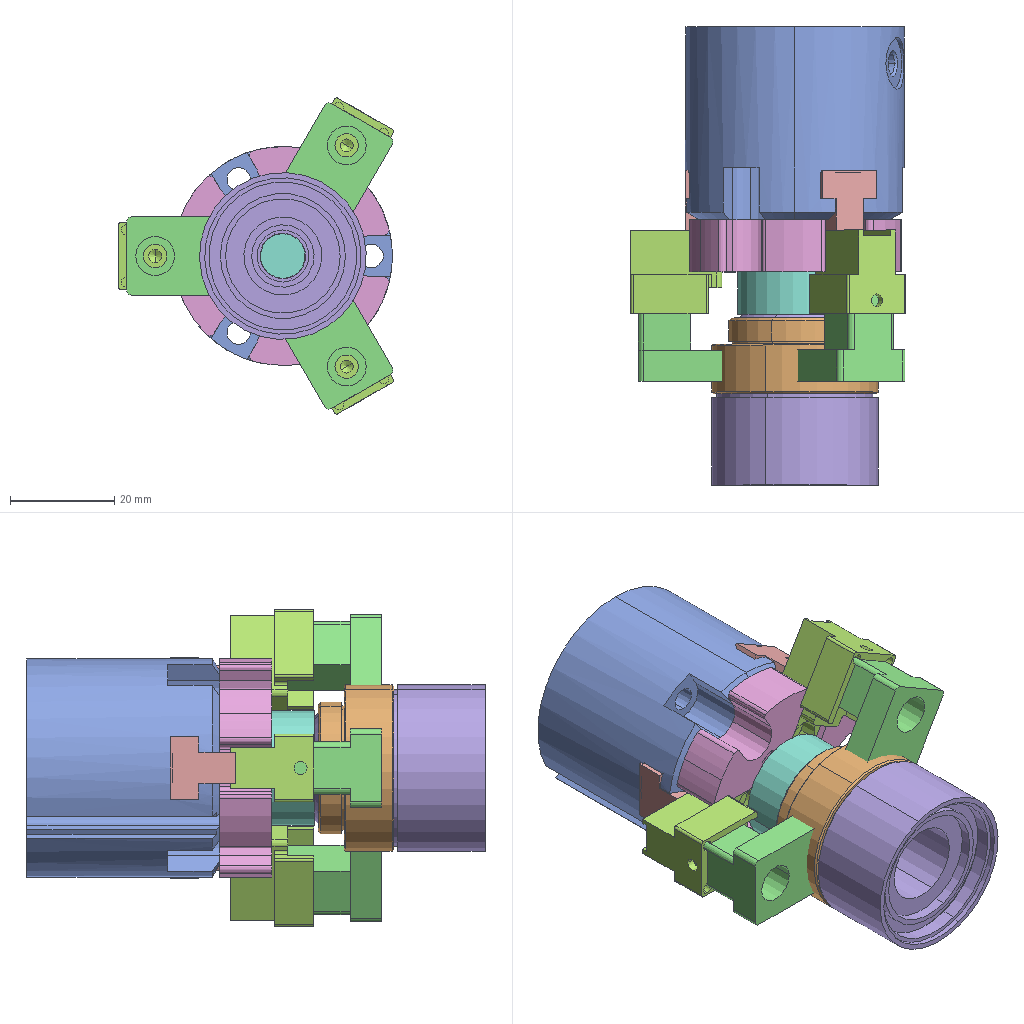Assembly | SolidWorks | 7 different items | 13 placed | box 53 x 88 x 61 mm
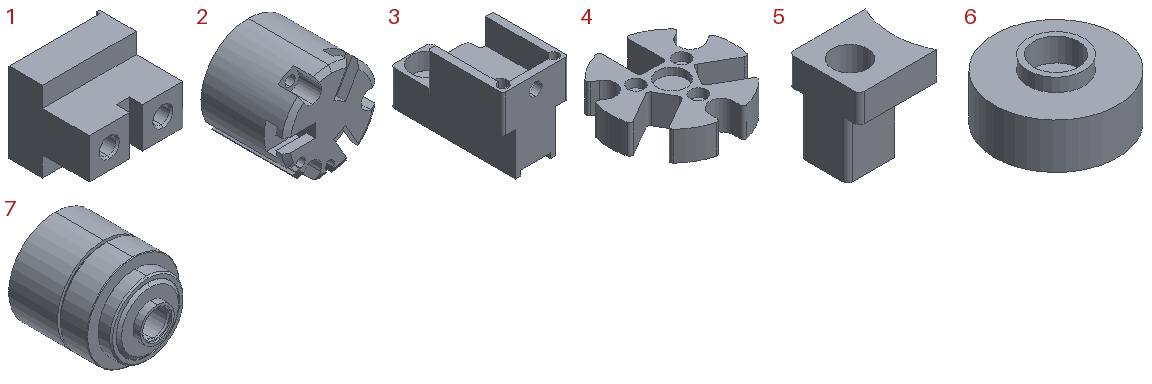Parts list (item | quantity | size | volume | features):
1 | x3 | 14 x 12.5 x 12 mm | 1347 mm3 | features BaseBody 1
2 | x1 | 42 x 37 x 41.953 mm | 41589 mm3 | features BaseBody 1
3 | x3 | 13 x 25 x 16 mm | 2086 mm3 | features ICE 9, Fillet 3, HoleWzd 3, Extrusion 1
4 | x1 | 42 x 40.594 x 10 mm | 7724 mm3 | features CirPattern 3, ICE 3, Fillet 2, Extrusion 1, HoleWzd 1
5 | x3 | 16.367 x 15 x 18 mm | 2039 mm3 | features ICE 3, Fillet 2, Extrusion 1, HoleWzd 1, MirrorPattern 1
6 | x1 | 22 x 22 x 10.5 mm | 2336 mm3 | features ICE 3, Chamfer 1, Extrusion 1
7 | x1 | 32 x 35.3 x 32 mm | 16584 mm3 | features Revolution 1
Mates (type | each side: item.copy, entity, surface, feature):
Width | 2.1 face plane MHS3-25D(0)_BODY | 2.1 face plane MHS3-25D(0)_BODY | 1.1 face plane MHS3-25(0)_FINGER | 1.1 face plane MHS3-25(0)_FINGER
Coincident | 1.1 face plane MHS3-25(0)_FINGER | 2.1 face plane MHS3-25D(0)_BODY
LimitDistanceDim | 1.1 face plane MHS3-25(0)_FINGER | 2.1 face plane MHS3-25D(0)_BODY
Coincident | 1.2 face plane MHS3-25(0)_FINGER | 3.1 face plane Cut-Extrude4
Concentric | 1.2 face cylinder MHS3-25(0)_FINGER | 3.1 face cylinder CBORE for M3 Hex Socket Head Cap Screw2
Width | 3.1 face plane Cut-Extrude4 | 3.1 face plane Cut-Extrude4 | 1.2 face plane MHS3-25(0)_FINGER | 1.2 face plane MHS3-25(0)_FINGER
Coincident | 2.1 face plane MHS3-25D(0)_BODY | 4.1 face plane Boss-Extrude1
Width | 4.1 face plane CirPattern1 | 4.1 face plane CirPattern1 | 3.2 face plane Cut-Extrude1 | 3.2 face plane Cut-Extrude1
Concentric | 2.1 edge | 4.1 edge
Concentric | 4.1 face cylinder Cut-Extrude4 | 6.1 face cylinder Cut-Extrude2
Coincident | 4.1 face plane Boss-Extrude1 | 6.1 face plane Cut-Extrude1
Concentric | 6.1 face cylinder Cut-Extrude3 | 7.1 face cylinder Revolve1
Coincident | 6.1 face plane Boss-Extrude1 | 7.1 face plane Revolve1
Concentric | 3.1 face cylinder M3 Tapped Hole1 | 5.1 face cylinder CBORE for M4 Hex Socket Head Cap Screw1
Width | 3.1 face plane Cut-Extrude11 | 3.1 face plane Cut-Extrude11 | 5.1 face plane Boss-Extrude1 | 5.1 face plane Boss-Extrude1
Coincident | 3.1 face plane Boss-Extrude5 | 5.1 face plane Boss-Extrude1